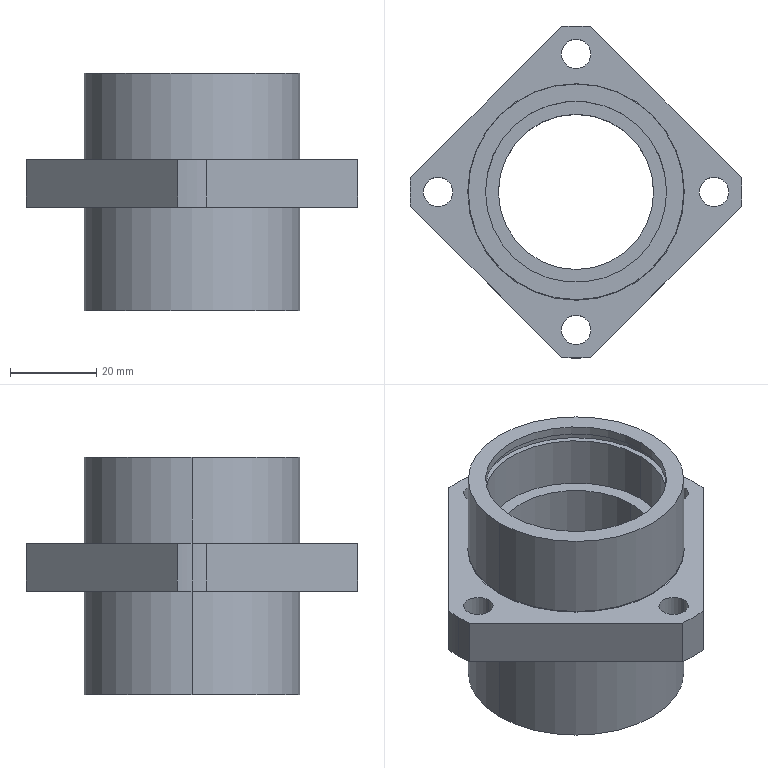Part | STEP file | BFU71-6004ZZ-L55-S20-001^BFU71-6004ZZ-L55-S20_Drive roller assembly | 1 solid | 59 faces | box 77 x 77 x 55 mm | volume 52767 mm3 | cylinder 39 | plane 18 | torus 2 | commonest cylinder face diameters 6.8 x8 11 x8 42 x8 77 x5 44.5 x4 50 x4